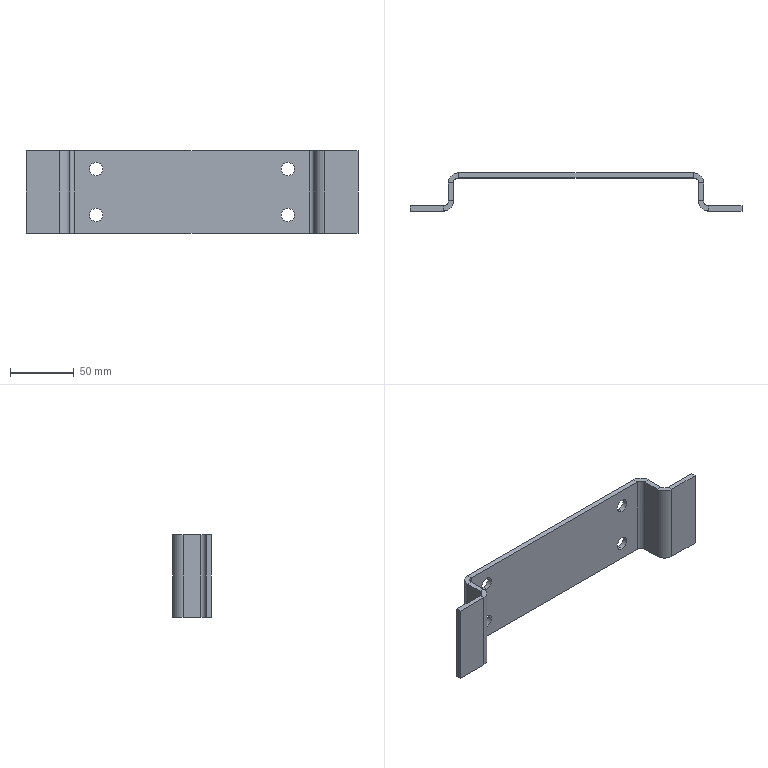Part | SolidWorks | features FlatPattern 1, ICE 1, SMBaseFlange 1, SheetMetal 1 | 1 solid | 46 faces | box 260 x 30 x 64.5 mm | volume 76453 mm3 | plane 30 | cylinder 16 | commonest cylinder face diameters 10.5 x8 8 x4 16 x4
STEP:
#1=CARTESIAN_POINT('',(-75.,-4.,23.25));
#2=VERTEX_POINT('',#1);
#3=CARTESIAN_POINT('',(-75.,-4.,12.75));
#4=VERTEX_POINT('',#3);
#5=CARTESIAN_POINT('',(-75.,-4.,18.));
#6=DIRECTION('',(0.,-1.,0.));
#7=DIRECTION('',(0.,0.,1.));
#8=AXIS2_PLACEMENT_3D('',#5,#6,#7);
#9=CIRCLE('',#8,5.25);
#10=EDGE_CURVE('',#2,#4,#9,.T.);
#11=ORIENTED_EDGE('',*,*,#10,.T.);
#12=CARTESIAN_POINT('',(-75.,0.,12.75));
#13=VERTEX_POINT('',#12);
#14=CARTESIAN_POINT('',(-75.,-30.001,12.75));
#15=DIRECTION('',(0.,1.,0.));
#16=VECTOR('',#15,1000.);
#17=LINE('',#14,#16);
#18=EDGE_CURVE('',#4,#13,#17,.T.);
#19=ORIENTED_EDGE('',*,*,#18,.T.);
#20=CARTESIAN_POINT('',(-75.,0.,23.25));
#21=VERTEX_POINT('',#20);
#22=CARTESIAN_POINT('',(-75.,0.,18.));
#23=DIRECTION('',(0.,1.,0.));
#24=DIRECTION('',(0.,0.,1.));
#25=AXIS2_PLACEMENT_3D('',#22,#23,#24);
#26=CIRCLE('',#25,5.25);
#27=EDGE_CURVE('',#13,#21,#26,.T.);
#28=ORIENTED_EDGE('',*,*,#27,.T.);
#29=CARTESIAN_POINT('',(-75.,-30.001,23.25));
#30=DIRECTION('',(0.,1.,0.));
#31=VECTOR('',#30,1000.);
#32=LINE('',#29,#31);
#33=EDGE_CURVE('',#2,#21,#32,.T.);
#34=ORIENTED_EDGE('',*,*,#33,.F.);
#35=EDGE_LOOP('',(#11,#19,#28,#34));
#36=FACE_OUTER_BOUND('',#35,.T.);
#37=CARTESIAN_POINT('',(-75.,-30.001,18.));
#38=DIRECTION('',(0.,1.,0.));
#39=DIRECTION('',(0.,0.,1.));
#40=AXIS2_PLACEMENT_3D('',#37,#38,#39);
#41=CYLINDRICAL_SURFACE('',#40,5.25);
#42=ADVANCED_FACE('',(#36),#41,.F.);
#43=CARTESIAN_POINT('',(75.,-4.,-12.75));
#44=VERTEX_POINT('',#43);
#45=CARTESIAN_POINT('',(75.,-4.,-23.25));
#46=VERTEX_POINT('',#45);
#47=CARTESIAN_POINT('',(75.,-4.,-18.));
#48=DIRECTION('',(0.,-1.,0.));
#49=DIRECTION('',(0.,0.,1.));
#50=AXIS2_PLACEMENT_3D('',#47,#48,#49);
#51=CIRCLE('',#50,5.25);
#52=EDGE_CURVE('',#44,#46,#51,.T.);
#53=ORIENTED_EDGE('',*,*,#52,.T.);
#54=CARTESIAN_POINT('',(75.,0.,-23.25));
#55=VERTEX_POINT('',#54);
#56=CARTESIAN_POINT('',(75.,-30.001,-23.25));
#57=DIRECTION('',(0.,1.,0.));
#58=VECTOR('',#57,1000.);
#59=LINE('',#56,#58);
#60=EDGE_CURVE('',#46,#55,#59,.T.);
#61=ORIENTED_EDGE('',*,*,#60,.T.);
#62=CARTESIAN_POINT('',(75.,0.,-12.75));
#63=VERTEX_POINT('',#62);
#64=CARTESIAN_POINT('',(75.,0.,-18.));
#65=DIRECTION('',(0.,1.,0.));
#66=DIRECTION('',(0.,0.,1.));
#67=AXIS2_PLACEMENT_3D('',#64,#65,#66);
#68=CIRCLE('',#67,5.25);
#69=EDGE_CURVE('',#55,#63,#68,.T.);
#70=ORIENTED_EDGE('',*,*,#69,.T.);
#71=CARTESIAN_POINT('',(75.,-30.001,-12.75));
#72=DIRECTION('',(0.,1.,0.));
#73=VECTOR('',#72,1000.);
#74=LINE('',#71,#73);
#75=EDGE_CURVE('',#44,#63,#74,.T.);
#76=ORIENTED_EDGE('',*,*,#75,.F.);
#77=EDGE_LOOP('',(#53,#61,#70,#76));
#78=FACE_OUTER_BOUND('',#77,.T.);
#79=CARTESIAN_POINT('',(75.,-30.001,-18.));
#80=DIRECTION('',(0.,1.,0.));
#81=DIRECTION('',(0.,0.,1.));
#82=AXIS2_PLACEMENT_3D('',#79,#80,#81);
#83=CYLINDRICAL_SURFACE('',#82,5.25);
#84=ADVANCED_FACE('',(#78),#83,.F.);
#85=CARTESIAN_POINT('',(75.,-4.,23.25));
#86=VERTEX_POINT('',#85);
#87=CARTESIAN_POINT('',(75.,-4.,12.75));
#88=VERTEX_POINT('',#87);
#89=CARTESIAN_POINT('',(75.,-4.,18.));
#90=DIRECTION('',(0.,-1.,0.));
#91=DIRECTION('',(0.,0.,1.));
#92=AXIS2_PLACEMENT_3D('',#89,#90,#91);
#93=CIRCLE('',#92,5.25);
#94=EDGE_CURVE('',#86,#88,#93,.T.);
#95=ORIENTED_EDGE('',*,*,#94,.T.);
#96=CARTESIAN_POINT('',(75.,0.,12.75));
#97=VERTEX_POINT('',#96);
#98=CARTESIAN_POINT('',(75.,-30.001,12.75));
#99=DIRECTION('',(0.,1.,0.));
#100=VECTOR('',#99,1000.);
#101=LINE('',#98,#100);
#102=EDGE_CURVE('',#88,#97,#101,.T.);
#103=ORIENTED_EDGE('',*,*,#102,.T.);
#104=CARTESIAN_POINT('',(75.,0.,23.25));
#105=VERTEX_POINT('',#104);
#106=CARTESIAN_POINT('',(75.,0.,18.));
#107=DIRECTION('',(0.,1.,0.));
#108=DIRECTION('',(0.,0.,1.));
#109=AXIS2_PLACEMENT_3D('',#106,#107,#108);
#110=CIRCLE('',#109,5.25);
#111=EDGE_CURVE('',#97,#105,#110,.T.);
#112=ORIENTED_EDGE('',*,*,#111,.T.);
#113=CARTESIAN_POINT('',(75.,-30.001,23.25));
#114=DIRECTION('',(0.,1.,0.));
#115=VECTOR('',#114,1000.);
#116=LINE('',#113,#115);
#117=EDGE_CURVE('',#86,#105,#116,.T.);
#118=ORIENTED_EDGE('',*,*,#117,.F.);
#119=EDGE_LOOP('',(#95,#103,#112,#118));
#120=FACE_OUTER_BOUND('',#119,.T.);
#121=CARTESIAN_POINT('',(75.,-30.001,18.));
#122=DIRECTION('',(0.,1.,0.));
#123=DIRECTION('',(0.,0.,1.));
#124=AXIS2_PLACEMENT_3D('',#121,#122,#123);
#125=CYLINDRICAL_SURFACE('',#124,5.25);
#126=ADVANCED_FACE('',(#120),#125,.F.);
#127=CARTESIAN_POINT('',(-75.,-4.,-12.75));
#128=VERTEX_POINT('',#127);
#129=CARTESIAN_POINT('',(-75.,-4.,-23.25));
#130=VERTEX_POINT('',#129);
#131=CARTESIAN_POINT('',(-75.,-4.,-18.));
#132=DIRECTION('',(0.,-1.,0.));
#133=DIRECTION('',(0.,0.,1.));
#134=AXIS2_PLACEMENT_3D('',#131,#132,#133);
#135=CIRCLE('',#134,5.25);
#136=EDGE_CURVE('',#128,#130,#135,.T.);
#137=ORIENTED_EDGE('',*,*,#136,.T.);
#138=CARTESIAN_POINT('',(-75.,0.,-23.25));
#139=VERTEX_POINT('',#138);
#140=CARTESIAN_POINT('',(-75.,-30.001,-23.25));
#141=DIRECTION('',(0.,1.,0.));
#142=VECTOR('',#141,1000.);
#143=LINE('',#140,#142);
#144=EDGE_CURVE('',#130,#139,#143,.T.);
#145=ORIENTED_EDGE('',*,*,#144,.T.);
#146=CARTESIAN_POINT('',(-75.,0.,-12.75));
#147=VERTEX_POINT('',#146);
#148=CARTESIAN_POINT('',(-75.,0.,-18.));
#149=DIRECTION('',(0.,1.,0.));
#150=DIRECTION('',(0.,0.,1.));
#151=AXIS2_PLACEMENT_3D('',#148,#149,#150);
#152=CIRCLE('',#151,5.25);
#153=EDGE_CURVE('',#139,#147,#152,.T.);
#154=ORIENTED_EDGE('',*,*,#153,.T.);
#155=CARTESIAN_POINT('',(-75.,-30.001,-12.75));
#156=DIRECTION('',(0.,1.,0.));
#157=VECTOR('',#156,1000.);
#158=LINE('',#155,#157);
#159=EDGE_CURVE('',#128,#147,#158,.T.);
#160=ORIENTED_EDGE('',*,*,#159,.F.);
#161=EDGE_LOOP('',(#137,#145,#154,#160));
#162=FACE_OUTER_BOUND('',#161,.T.);
#163=CARTESIAN_POINT('',(-75.,-30.001,-18.));
#164=DIRECTION('',(0.,1.,0.));
#165=DIRECTION('',(0.,0.,1.));
#166=AXIS2_PLACEMENT_3D('',#163,#164,#165);
#167=CYLINDRICAL_SURFACE('',#166,5.25);
#168=ADVANCED_FACE('',(#162),#167,.F.);
#169=CARTESIAN_POINT('',(-100.,-22.,32.25));
#170=VERTEX_POINT('',#169);
#171=CARTESIAN_POINT('',(-96.,-22.,32.25));
#172=VERTEX_POINT('',#171);
#173=CARTESIAN_POINT('',(-100.,-22.,32.25));
#174=DIRECTION('',(1.,0.,0.));
#175=VECTOR('',#174,1000.);
#176=LINE('',#173,#175);
#177=EDGE_CURVE('',#170,#172,#176,.T.);
#178=ORIENTED_EDGE('',*,*,#177,.F.);
#179=CARTESIAN_POINT('',(-104.,-26.,32.25));
#180=VERTEX_POINT('',#179);
#181=CARTESIAN_POINT('',(-104.,-22.,32.25));
#182=DIRECTION('',(0.,0.,1.));
#183=DIRECTION('',(-1.,0.,0.));
#184=AXIS2_PLACEMENT_3D('',#181,#182,#183);
#185=CIRCLE('',#184,4.);
#186=EDGE_CURVE('',#180,#170,#185,.T.);
#187=ORIENTED_EDGE('',*,*,#186,.F.);
#188=CARTESIAN_POINT('',(-104.,-30.,32.25));
#189=VERTEX_POINT('',#188);
#190=CARTESIAN_POINT('',(-104.,-30.,32.25));
#191=DIRECTION('',(0.,1.,0.));
#192=VECTOR('',#191,1000.);
#193=LINE('',#190,#192);
#194=EDGE_CURVE('',#189,#180,#193,.T.);
#195=ORIENTED_EDGE('',*,*,#194,.F.);
#196=CARTESIAN_POINT('',(-104.,-22.,32.25));
#197=DIRECTION('',(0.,0.,1.));
#198=DIRECTION('',(1.,0.,0.));
#199=AXIS2_PLACEMENT_3D('',#196,#197,#198);
#200=CIRCLE('',#199,8.);
#201=EDGE_CURVE('',#189,#172,#200,.T.);
#202=ORIENTED_EDGE('',*,*,#201,.T.);
#203=EDGE_LOOP('',(#178,#187,#195,#202));
#204=FACE_OUTER_BOUND('',#203,.T.);
#205=CARTESIAN_POINT('',(-100.,-22.,32.25));
#206=DIRECTION('',(0.,0.,1.));
#207=DIRECTION('',(1.,0.,0.));
#208=AXIS2_PLACEMENT_3D('',#205,#206,#207);
#209=PLANE('',#208);
#210=ADVANCED_FACE('',(#204),#209,.T.);
#211=CARTESIAN_POINT('',(-100.,-8.,32.25));
#212=VERTEX_POINT('',#211);
#213=CARTESIAN_POINT('',(-100.,-26.,32.25));
#214=DIRECTION('',(0.,1.,0.));
#215=VECTOR('',#214,1000.);
#216=LINE('',#213,#215);
#217=EDGE_CURVE('',#170,#212,#216,.T.);
#218=ORIENTED_EDGE('',*,*,#217,.F.);
#219=ORIENTED_EDGE('',*,*,#177,.T.);
#220=CARTESIAN_POINT('',(-96.,-8.,32.25));
#221=VERTEX_POINT('',#220);
#222=CARTESIAN_POINT('',(-96.,-26.,32.25));
#223=DIRECTION('',(0.,1.,0.));
#224=VECTOR('',#223,1000.);
#225=LINE('',#222,#224);
#226=EDGE_CURVE('',#172,#221,#225,.T.);
#227=ORIENTED_EDGE('',*,*,#226,.T.);
#228=CARTESIAN_POINT('',(-96.,-8.,32.25));
#229=DIRECTION('',(-1.,0.,0.));
#230=VECTOR('',#229,1000.);
#231=LINE('',#228,#230);
#232=EDGE_CURVE('',#221,#212,#231,.T.);
#233=ORIENTED_EDGE('',*,*,#232,.T.);
#234=EDGE_LOOP('',(#218,#219,#227,#233));
#235=FACE_OUTER_BOUND('',#234,.T.);
#236=CARTESIAN_POINT('',(-104.,-30.,32.25));
#237=DIRECTION('',(0.,0.,1.));
#238=DIRECTION('',(1.,0.,0.));
#239=AXIS2_PLACEMENT_3D('',#236,#237,#238);
#240=PLANE('',#239);
#241=ADVANCED_FACE('',(#235),#240,.T.);
#242=CARTESIAN_POINT('',(-104.,-26.,-32.25));
#243=VERTEX_POINT('',#242);
#244=CARTESIAN_POINT('',(-104.,-30.,-32.25));
#245=VERTEX_POINT('',#244);
#246=CARTESIAN_POINT('',(-104.,-26.,-32.25));
#247=DIRECTION('',(0.,-1.,0.));
#248=VECTOR('',#247,1000.);
#249=LINE('',#246,#248);
#250=EDGE_CURVE('',#243,#245,#249,.T.);
#251=ORIENTED_EDGE('',*,*,#250,.F.);
#252=CARTESIAN_POINT('',(-100.,-22.,-32.25));
#253=VERTEX_POINT('',#252);
#254=CARTESIAN_POINT('',(-104.,-22.,-32.25));
#255=DIRECTION('',(0.,0.,1.));
#256=DIRECTION('',(-1.,0.,0.));
#257=AXIS2_PLACEMENT_3D('',#254,#255,#256);
#258=CIRCLE('',#257,4.);
#259=EDGE_CURVE('',#243,#253,#258,.T.);
#260=ORIENTED_EDGE('',*,*,#259,.T.);
#261=CARTESIAN_POINT('',(-96.,-22.,-32.25));
#262=VERTEX_POINT('',#261);
#263=CARTESIAN_POINT('',(-96.,-22.,-32.25));
#264=DIRECTION('',(-1.,0.,0.));
#265=VECTOR('',#264,1000.);
#266=LINE('',#263,#265);
#267=EDGE_CURVE('',#262,#253,#266,.T.);
#268=ORIENTED_EDGE('',*,*,#267,.F.);
#269=CARTESIAN_POINT('',(-104.,-22.,-32.25));
#270=DIRECTION('',(0.,0.,1.));
#271=DIRECTION('',(1.,0.,0.));
#272=AXIS2_PLACEMENT_3D('',#269,#270,#271);
#273=CIRCLE('',#272,8.);
#274=EDGE_CURVE('',#245,#262,#273,.T.);
#275=ORIENTED_EDGE('',*,*,#274,.F.);
#276=EDGE_LOOP('',(#251,#260,#268,#275));
#277=FACE_OUTER_BOUND('',#276,.T.);
#278=CARTESIAN_POINT('',(-104.,-26.,-32.25));
#279=DIRECTION('',(0.,0.,-1.));
#280=DIRECTION('',(-1.,0.,0.));
#281=AXIS2_PLACEMENT_3D('',#278,#279,#280);
#282=PLANE('',#281);
#283=ADVANCED_FACE('',(#277),#282,.T.);
#284=CARTESIAN_POINT('',(-130.,-26.,-32.25));
#285=VERTEX_POINT('',#284);
#286=CARTESIAN_POINT('',(-130.,-26.,-32.25));
#287=DIRECTION('',(1.,0.,0.));
#288=VECTOR('',#287,1000.);
#289=LINE('',#286,#288);
#290=EDGE_CURVE('',#285,#243,#289,.T.);
#291=ORIENTED_EDGE('',*,*,#290,.T.);
#292=ORIENTED_EDGE('',*,*,#250,.T.);
#293=CARTESIAN_POINT('',(-130.,-30.,-32.25));
#294=VERTEX_POINT('',#293);
#295=CARTESIAN_POINT('',(-130.,-30.,-32.25));
#296=DIRECTION('',(1.,0.,0.));
#297=VECTOR('',#296,1000.);
#298=LINE('',#295,#297);
#299=EDGE_CURVE('',#294,#245,#298,.T.);
#300=ORIENTED_EDGE('',*,*,#299,.F.);
#301=CARTESIAN_POINT('',(-130.,-30.,-32.25));
#302=DIRECTION('',(0.,1.,0.));
#303=VECTOR('',#302,1000.);
#304=LINE('',#301,#303);
#305=EDGE_CURVE('',#294,#285,#304,.T.);
#306=ORIENTED_EDGE('',*,*,#305,.T.);
#307=EDGE_LOOP('',(#291,#292,#300,#306));
#308=FACE_OUTER_BOUND('',#307,.T.);
#309=CARTESIAN_POINT('',(-96.,-22.,-32.25));
#310=DIRECTION('',(0.,0.,-1.));
#311=DIRECTION('',(-1.,0.,0.));
#312=AXIS2_PLACEMENT_3D('',#309,#310,#311);
#313=PLANE('',#312);
#314=ADVANCED_FACE('',(#308),#313,.T.);
#315=CARTESIAN_POINT('',(-92.,0.,32.25));
#316=VERTEX_POINT('',#315);
#317=CARTESIAN_POINT('',(-92.,-4.,32.25));
#318=VERTEX_POINT('',#317);
#319=CARTESIAN_POINT('',(-92.,0.,32.25));
#320=DIRECTION('',(0.,-1.,0.));
#321=VECTOR('',#320,1000.);
#322=LINE('',#319,#321);
#323=EDGE_CURVE('',#316,#318,#322,.T.);
#324=ORIENTED_EDGE('',*,*,#323,.F.);
#325=CARTESIAN_POINT('',(-92.,-8.,32.25));
#326=DIRECTION('',(0.,0.,-1.));
#327=DIRECTION('',(1.,0.,0.));
#328=AXIS2_PLACEMENT_3D('',#325,#326,#327);
#329=CIRCLE('',#328,8.);
#330=EDGE_CURVE('',#212,#316,#329,.T.);
#331=ORIENTED_EDGE('',*,*,#330,.F.);
#332=ORIENTED_EDGE('',*,*,#232,.F.);
#333=CARTESIAN_POINT('',(-92.,-8.,32.25));
#334=DIRECTION('',(0.,0.,-1.));
#335=DIRECTION('',(1.,0.,0.));
#336=AXIS2_PLACEMENT_3D('',#333,#334,#335);
#337=CIRCLE('',#336,4.);
#338=EDGE_CURVE('',#221,#318,#337,.T.);
#339=ORIENTED_EDGE('',*,*,#338,.T.);
#340=EDGE_LOOP('',(#324,#331,#332,#339));
#341=FACE_OUTER_BOUND('',#340,.T.);
#342=CARTESIAN_POINT('',(-92.,0.,32.25));
#343=DIRECTION('',(0.,0.,1.));
#344=DIRECTION('',(1.,0.,0.));
#345=AXIS2_PLACEMENT_3D('',#342,#343,#344);
#346=PLANE('',#345);
#347=ADVANCED_FACE('',(#341),#346,.T.);
#348=CARTESIAN_POINT('',(92.,0.,32.25));
#349=VERTEX_POINT('',#348);
#350=CARTESIAN_POINT('',(-100.,0.,32.25));
#351=DIRECTION('',(1.,0.,0.));
#352=VECTOR('',#351,1000.);
#353=LINE('',#350,#352);
#354=EDGE_CURVE('',#316,#349,#353,.T.);
#355=ORIENTED_EDGE('',*,*,#354,.F.);
#356=ORIENTED_EDGE('',*,*,#323,.T.);
#357=CARTESIAN_POINT('',(92.,-4.,32.25));
#358=VERTEX_POINT('',#357);
#359=CARTESIAN_POINT('',(-100.,-4.,32.25));
#360=DIRECTION('',(1.,0.,0.));
#361=VECTOR('',#360,1000.);
#362=LINE('',#359,#361);
#363=EDGE_CURVE('',#318,#358,#362,.T.);
#364=ORIENTED_EDGE('',*,*,#363,.T.);
#365=CARTESIAN_POINT('',(92.,-4.,32.25));
#366=DIRECTION('',(0.,1.,0.));
#367=VECTOR('',#366,1000.);
#368=LINE('',#365,#367);
#369=EDGE_CURVE('',#358,#349,#368,.T.);
#370=ORIENTED_EDGE('',*,*,#369,.T.);
#371=EDGE_LOOP('',(#355,#356,#364,#370));
#372=FACE_OUTER_BOUND('',#371,.T.);
#373=CARTESIAN_POINT('',(-96.,-8.,32.25));
#374=DIRECTION('',(0.,0.,1.));
#375=DIRECTION('',(1.,0.,0.));
#376=AXIS2_PLACEMENT_3D('',#373,#374,#375);
#377=PLANE('',#376);
#378=ADVANCED_FACE('',(#372),#377,.T.);
#379=CARTESIAN_POINT('',(-100.,-8.,-32.25));
#380=VERTEX_POINT('',#379);
#381=CARTESIAN_POINT('',(-96.,-8.,-32.25));
#382=VERTEX_POINT('',#381);
#383=CARTESIAN_POINT('',(-100.,-8.,-32.25));
#384=DIRECTION('',(1.,0.,0.));
#385=VECTOR('',#384,1000.);
#386=LINE('',#383,#385);
#387=EDGE_CURVE('',#380,#382,#386,.T.);
#388=ORIENTED_EDGE('',*,*,#387,.F.);
#389=CARTESIAN_POINT('',(-92.,0.,-32.25));
#390=VERTEX_POINT('',#389);
#391=CARTESIAN_POINT('',(-92.,-8.,-32.25));
#392=DIRECTION('',(0.,0.,-1.));
#393=DIRECTION('',(1.,0.,0.));
#394=AXIS2_PLACEMENT_3D('',#391,#392,#393);
#395=CIRCLE('',#394,8.);
#396=EDGE_CURVE('',#380,#390,#395,.T.);
#397=ORIENTED_EDGE('',*,*,#396,.T.);
#398=CARTESIAN_POINT('',(-92.,-4.,-32.25));
#399=VERTEX_POINT('',#398);
#400=CARTESIAN_POINT('',(-92.,-4.,-32.25));
#401=DIRECTION('',(0.,1.,0.));
#402=VECTOR('',#401,1000.);
#403=LINE('',#400,#402);
#404=EDGE_CURVE('',#399,#390,#403,.T.);
#405=ORIENTED_EDGE('',*,*,#404,.F.);
#406=CARTESIAN_POINT('',(-92.,-8.,-32.25));
#407=DIRECTION('',(0.,0.,-1.));
#408=DIRECTION('',(1.,0.,0.));
#409=AXIS2_PLACEMENT_3D('',#406,#407,#408);
#410=CIRCLE('',#409,4.);
#411=EDGE_CURVE('',#382,#399,#410,.T.);
#412=ORIENTED_EDGE('',*,*,#411,.F.);
#413=EDGE_LOOP('',(#388,#397,#405,#412));
#414=FACE_OUTER_BOUND('',#413,.T.);
#415=CARTESIAN_POINT('',(-100.,-8.,-32.25));
#416=DIRECTION('',(0.,0.,-1.));
#417=DIRECTION('',(-1.,0.,0.));
#418=AXIS2_PLACEMENT_3D('',#415,#416,#417);
#419=PLANE('',#418);
#420=ADVANCED_FACE('',(#414),#419,.T.);
#421=CARTESIAN_POINT('',(-100.,-26.,-32.25));
#422=DIRECTION('',(0.,1.,0.));
#423=VECTOR('',#422,1000.);
#424=LINE('',#421,#423);
#425=EDGE_CURVE('',#253,#380,#424,.T.);
#426=ORIENTED_EDGE('',*,*,#425,.T.);
#427=ORIENTED_EDGE('',*,*,#387,.T.);
#428=CARTESIAN_POINT('',(-96.,-26.,-32.25));
#429=DIRECTION('',(0.,1.,0.));
#430=VECTOR('',#429,1000.);
#431=LINE('',#428,#430);
#432=EDGE_CURVE('',#262,#382,#431,.T.);
#433=ORIENTED_EDGE('',*,*,#432,.F.);
#434=ORIENTED_EDGE('',*,*,#267,.T.);
#435=EDGE_LOOP('',(#426,#427,#433,#434));
#436=FACE_OUTER_BOUND('',#435,.T.);
#437=CARTESIAN_POINT('',(-92.,-4.,-32.25));
#438=DIRECTION('',(0.,0.,-1.));
#439=DIRECTION('',(-1.,0.,0.));
#440=AXIS2_PLACEMENT_3D('',#437,#438,#439);
#441=PLANE('',#440);
#442=ADVANCED_FACE('',(#436),#441,.T.);
#443=CARTESIAN_POINT('',(100.,-8.,32.25));
#444=VERTEX_POINT('',#443);
#445=CARTESIAN_POINT('',(96.,-8.,32.25));
#446=VERTEX_POINT('',#445);
#447=CARTESIAN_POINT('',(100.,-8.,32.25));
#448=DIRECTION('',(-1.,0.,0.));
#449=VECTOR('',#448,1000.);
#450=LINE('',#447,#449);
#451=EDGE_CURVE('',#444,#446,#450,.T.);
#452=ORIENTED_EDGE('',*,*,#451,.F.);
#453=CARTESIAN_POINT('',(92.,-8.,32.25));
#454=DIRECTION('',(0.,0.,-1.));
#455=DIRECTION('',(1.,0.,0.));
#456=AXIS2_PLACEMENT_3D('',#453,#454,#455);
#457=CIRCLE('',#456,8.);
#458=EDGE_CURVE('',#349,#444,#457,.T.);
#459=ORIENTED_EDGE('',*,*,#458,.F.);
#460=ORIENTED_EDGE('',*,*,#369,.F.);
#461=CARTESIAN_POINT('',(92.,-8.,32.25));
#462=DIRECTION('',(0.,0.,-1.));
#463=DIRECTION('',(1.,0.,0.));
#464=AXIS2_PLACEMENT_3D('',#461,#462,#463);
#465=CIRCLE('',#464,4.);
#466=EDGE_CURVE('',#358,#446,#465,.T.);
#467=ORIENTED_EDGE('',*,*,#466,.T.);
#468=EDGE_LOOP('',(#452,#459,#460,#467));
#469=FACE_OUTER_BOUND('',#468,.T.);
#470=CARTESIAN_POINT('',(100.,-8.,32.25));
#471=DIRECTION('',(0.,0.,1.));
#472=DIRECTION('',(1.,0.,0.));
#473=AXIS2_PLACEMENT_3D('',#470,#471,#472);
#474=PLANE('',#473);
#475=ADVANCED_FACE('',(#469),#474,.T.);
#476=CARTESIAN_POINT('',(100.,-22.,32.25));
#477=VERTEX_POINT('',#476);
#478=CARTESIAN_POINT('',(100.,0.,32.25));
#479=DIRECTION('',(0.,-1.,0.));
#480=VECTOR('',#479,1000.);
#481=LINE('',#478,#480);
#482=EDGE_CURVE('',#444,#477,#481,.T.);
#483=ORIENTED_EDGE('',*,*,#482,.F.);
#484=ORIENTED_EDGE('',*,*,#451,.T.);
#485=CARTESIAN_POINT('',(96.,-22.,32.25));
#486=VERTEX_POINT('',#485);
#487=CARTESIAN_POINT('',(96.,0.,32.25));
#488=DIRECTION('',(0.,-1.,0.));
#489=VECTOR('',#488,1000.);
#490=LINE('',#487,#489);
#491=EDGE_CURVE('',#446,#486,#490,.T.);
#492=ORIENTED_EDGE('',*,*,#491,.T.);
#493=CARTESIAN_POINT('',(96.,-22.,32.25));
#494=DIRECTION('',(1.,0.,0.));
#495=VECTOR('',#494,1000.);
#496=LINE('',#493,#495);
#497=EDGE_CURVE('',#486,#477,#496,.T.);
#498=ORIENTED_EDGE('',*,*,#497,.T.);
#499=EDGE_LOOP('',(#483,#484,#492,#498));
#500=FACE_OUTER_BOUND('',#499,.T.);
#501=CARTESIAN_POINT('',(92.,-4.,32.25));
#502=DIRECTION('',(0.,0.,1.));
#503=DIRECTION('',(1.,0.,0.));
#504=AXIS2_PLACEMENT_3D('',#501,#502,#503);
#505=PLANE('',#504);
#506=ADVANCED_FACE('',(#500),#505,.T.);
#507=CARTESIAN_POINT('',(92.,0.,-32.25));
#508=VERTEX_POINT('',#507);
#509=CARTESIAN_POINT('',(92.,-4.,-32.25));
#510=VERTEX_POINT('',#509);
#511=CARTESIAN_POINT('',(92.,0.,-32.25));
#512=DIRECTION('',(0.,-1.,0.));
#513=VECTOR('',#512,1000.);
#514=LINE('',#511,#513);
#515=EDGE_CURVE('',#508,#510,#514,.T.);
#516=ORIENTED_EDGE('',*,*,#515,.F.);
#517=CARTESIAN_POINT('',(100.,-8.,-32.25));
#518=VERTEX_POINT('',#517);
#519=CARTESIAN_POINT('',(92.,-8.,-32.25));
#520=DIRECTION('',(0.,0.,-1.));
#521=DIRECTION('',(1.,0.,0.));
#522=AXIS2_PLACEMENT_3D('',#519,#520,#521);
#523=CIRCLE('',#522,8.);
#524=EDGE_CURVE('',#508,#518,#523,.T.);
#525=ORIENTED_EDGE('',*,*,#524,.T.);
#526=CARTESIAN_POINT('',(96.,-8.,-32.25));
#527=VERTEX_POINT('',#526);
#528=CARTESIAN_POINT('',(96.,-8.,-32.25));
#529=DIRECTION('',(1.,0.,0.));
#530=VECTOR('',#529,1000.);
#531=LINE('',#528,#530);
#532=EDGE_CURVE('',#527,#518,#531,.T.);
#533=ORIENTED_EDGE('',*,*,#532,.F.);
#534=CARTESIAN_POINT('',(92.,-8.,-32.25));
#535=DIRECTION('',(0.,0.,-1.));
#536=DIRECTION('',(1.,0.,0.));
#537=AXIS2_PLACEMENT_3D('',#534,#535,#536);
#538=CIRCLE('',#537,4.);
#539=EDGE_CURVE('',#510,#527,#538,.T.);
#540=ORIENTED_EDGE('',*,*,#539,.F.);
#541=EDGE_LOOP('',(#516,#525,#533,#540));
#542=FACE_OUTER_BOUND('',#541,.T.);
#543=CARTESIAN_POINT('',(92.,0.,-32.25));
#544=DIRECTION('',(0.,0.,-1.));
#545=DIRECTION('',(-1.,0.,0.));
#546=AXIS2_PLACEMENT_3D('',#543,#544,#545);
#547=PLANE('',#546);
#548=ADVANCED_FACE('',(#542),#547,.T.);
#549=CARTESIAN_POINT('',(-100.,0.,-32.25));
#550=DIRECTION('',(1.,0.,0.));
#551=VECTOR('',#550,1000.);
#552=LINE('',#549,#551);
#553=EDGE_CURVE('',#390,#508,#552,.T.);
#554=ORIENTED_EDGE('',*,*,#553,.T.);
#555=ORIENTED_EDGE('',*,*,#515,.T.);
#556=CARTESIAN_POINT('',(-100.,-4.,-32.25));
#557=DIRECTION('',(1.,0.,0.));
#558=VECTOR('',#557,1000.);
#559=LINE('',#556,#558);
#560=EDGE_CURVE('',#399,#510,#559,.T.);
#561=ORIENTED_EDGE('',*,*,#560,.F.);
#562=ORIENTED_EDGE('',*,*,#404,.T.);
#563=EDGE_LOOP('',(#554,#555,#561,#562));
#564=FACE_OUTER_BOUND('',#563,.T.);
#565=CARTESIAN_POINT('',(96.,-8.,-32.25));
#566=DIRECTION('',(0.,0.,-1.));
#567=DIRECTION('',(-1.,0.,0.));
#568=AXIS2_PLACEMENT_3D('',#565,#566,#567);
#569=PLANE('',#568);
#570=ADVANCED_FACE('',(#564),#569,.T.);
#571=CARTESIAN_POINT('',(104.,-26.,32.25));
#572=VERTEX_POINT('',#571);
#573=CARTESIAN_POINT('',(104.,-30.,32.25));
#574=VERTEX_POINT('',#573);
#575=CARTESIAN_POINT('',(104.,-26.,32.25));
#576=DIRECTION('',(0.,-1.,0.));
#577=VECTOR('',#576,1000.);
#578=LINE('',#575,#577);
#579=EDGE_CURVE('',#572,#574,#578,.T.);
#580=ORIENTED_EDGE('',*,*,#579,.F.);
#581=CARTESIAN_POINT('',(104.,-22.,32.25));
#582=DIRECTION('',(0.,0.,1.));
#583=DIRECTION('',(-1.,0.,0.));
#584=AXIS2_PLACEMENT_3D('',#581,#582,#583);
#585=CIRCLE('',#584,4.);
#586=EDGE_CURVE('',#477,#572,#585,.T.);
#587=ORIENTED_EDGE('',*,*,#586,.F.);
#588=ORIENTED_EDGE('',*,*,#497,.F.);
#589=CARTESIAN_POINT('',(104.,-22.,32.25));
#590=DIRECTION('',(0.,0.,1.));
#591=DIRECTION('',(1.,0.,0.));
#592=AXIS2_PLACEMENT_3D('',#589,#590,#591);
#593=CIRCLE('',#592,8.);
#594=EDGE_CURVE('',#486,#574,#593,.T.);
#595=ORIENTED_EDGE('',*,*,#594,.T.);
#596=EDGE_LOOP('',(#580,#587,#588,#595));
#597=FACE_OUTER_BOUND('',#596,.T.);
#598=CARTESIAN_POINT('',(104.,-26.,32.25));
#599=DIRECTION('',(0.,0.,1.));
#600=DIRECTION('',(1.,0.,0.));
#601=AXIS2_PLACEMENT_3D('',#598,#599,#600);
#602=PLANE('',#601);
#603=ADVANCED_FACE('',(#597),#602,.T.);
#604=CARTESIAN_POINT('',(130.,-26.,32.25));
#605=VERTEX_POINT('',#604);
#606=CARTESIAN_POINT('',(100.,-26.,32.25));
#607=DIRECTION('',(1.,0.,0.));
#608=VECTOR('',#607,1000.);
#609=LINE('',#606,#608);
#610=EDGE_CURVE('',#572,#605,#609,.T.);
#611=ORIENTED_EDGE('',*,*,#610,.F.);
#612=ORIENTED_EDGE('',*,*,#579,.T.);
#613=CARTESIAN_POINT('',(130.,-30.,32.25));
#614=VERTEX_POINT('',#613);
#615=CARTESIAN_POINT('',(100.,-30.,32.25));
#616=DIRECTION('',(1.,0.,0.));
#617=VECTOR('',#616,1000.);
#618=LINE('',#615,#617);
#619=EDGE_CURVE('',#574,#614,#618,.T.);
#620=ORIENTED_EDGE('',*,*,#619,.T.);
#621=CARTESIAN_POINT('',(130.,-26.,32.25));
#622=DIRECTION('',(0.,-1.,0.));
#623=VECTOR('',#622,1000.);
#624=LINE('',#621,#623);
#625=EDGE_CURVE('',#605,#614,#624,.T.);
#626=ORIENTED_EDGE('',*,*,#625,.F.);
#627=EDGE_LOOP('',(#611,#612,#620,#626));
#628=FACE_OUTER_BOUND('',#627,.T.);
#629=CARTESIAN_POINT('',(96.,-22.,32.25));
#630=DIRECTION('',(0.,0.,1.));
#631=DIRECTION('',(1.,0.,0.));
#632=AXIS2_PLACEMENT_3D('',#629,#630,#631);
#633=PLANE('',#632);
#634=ADVANCED_FACE('',(#628),#633,.T.);
#635=CARTESIAN_POINT('',(100.,-22.,-32.25));
#636=VERTEX_POINT('',#635);
#637=CARTESIAN_POINT('',(96.,-22.,-32.25));
#638=VERTEX_POINT('',#637);
#639=CARTESIAN_POINT('',(100.,-22.,-32.25));
#640=DIRECTION('',(-1.,0.,0.));
#641=VECTOR('',#640,1000.);
#642=LINE('',#639,#641);
#643=EDGE_CURVE('',#636,#638,#642,.T.);
#644=ORIENTED_EDGE('',*,*,#643,.F.);
#645=CARTESIAN_POINT('',(104.,-26.,-32.25));
#646=VERTEX_POINT('',#645);
#647=CARTESIAN_POINT('',(104.,-22.,-32.25));
#648=DIRECTION('',(0.,0.,1.));
#649=DIRECTION('',(-1.,0.,0.));
#650=AXIS2_PLACEMENT_3D('',#647,#648,#649);
#651=CIRCLE('',#650,4.);
#652=EDGE_CURVE('',#636,#646,#651,.T.);
#653=ORIENTED_EDGE('',*,*,#652,.T.);
#654=CARTESIAN_POINT('',(104.,-30.,-32.25));
#655=VERTEX_POINT('',#654);
#656=CARTESIAN_POINT('',(104.,-30.,-32.25));
#657=DIRECTION('',(0.,1.,0.));
#658=VECTOR('',#657,1000.);
#659=LINE('',#656,#658);
#660=EDGE_CURVE('',#655,#646,#659,.T.);
#661=ORIENTED_EDGE('',*,*,#660,.F.);
#662=CARTESIAN_POINT('',(104.,-22.,-32.25));
#663=DIRECTION('',(0.,0.,1.));
#664=DIRECTION('',(1.,0.,0.));
#665=AXIS2_PLACEMENT_3D('',#662,#663,#664);
#666=CIRCLE('',#665,8.);
#667=EDGE_CURVE('',#638,#655,#666,.T.);
#668=ORIENTED_EDGE('',*,*,#667,.F.);
#669=EDGE_LOOP('',(#644,#653,#661,#668));
#670=FACE_OUTER_BOUND('',#669,.T.);
#671=CARTESIAN_POINT('',(100.,-22.,-32.25));
#672=DIRECTION('',(0.,0.,-1.));
#673=DIRECTION('',(-1.,0.,0.));
#674=AXIS2_PLACEMENT_3D('',#671,#672,#673);
#675=PLANE('',#674);
#676=ADVANCED_FACE('',(#670),#675,.T.);
#677=CARTESIAN_POINT('',(100.,0.,-32.25));
#678=DIRECTION('',(0.,-1.,0.));
#679=VECTOR('',#678,1000.);
#680=LINE('',#677,#679);
#681=EDGE_CURVE('',#518,#636,#680,.T.);
#682=ORIENTED_EDGE('',*,*,#681,.T.);
#683=ORIENTED_EDGE('',*,*,#643,.T.);
#684=CARTESIAN_POINT('',(96.,0.,-32.25));
#685=DIRECTION('',(0.,-1.,0.));
#686=VECTOR('',#685,1000.);
#687=LINE('',#684,#686);
#688=EDGE_CURVE('',#527,#638,#687,.T.);
#689=ORIENTED_EDGE('',*,*,#688,.F.);
#690=ORIENTED_EDGE('',*,*,#532,.T.);
#691=EDGE_LOOP('',(#682,#683,#689,#690));
#692=FACE_OUTER_BOUND('',#691,.T.);
#693=CARTESIAN_POINT('',(104.,-30.,-32.25));
#694=DIRECTION('',(0.,0.,-1.));
#695=DIRECTION('',(-1.,0.,0.));
#696=AXIS2_PLACEMENT_3D('',#693,#694,#695);
#697=PLANE('',#696);
#698=ADVANCED_FACE('',(#692),#697,.T.);
#699=CARTESIAN_POINT('',(130.,-30.,-32.25));
#700=VERTEX_POINT('',#699);
#701=CARTESIAN_POINT('',(100.,-30.,-32.25));
#702=DIRECTION('',(1.,0.,0.));
#703=VECTOR('',#702,1000.);
#704=LINE('',#701,#703);
#705=EDGE_CURVE('',#655,#700,#704,.T.);
#706=ORIENTED_EDGE('',*,*,#705,.T.);
#707=CARTESIAN_POINT('',(130.,-30.,32.25));
#708=DIRECTION('',(0.,0.,-1.));
#709=VECTOR('',#708,1000.);
#710=LINE('',#707,#709);
#711=EDGE_CURVE('',#614,#700,#710,.T.);
#712=ORIENTED_EDGE('',*,*,#711,.F.);
#713=ORIENTED_EDGE('',*,*,#619,.F.);
#714=CARTESIAN_POINT('',(104.,-30.,32.25));
#715=DIRECTION('',(0.,0.,-1.));
#716=VECTOR('',#715,1000.);
#717=LINE('',#714,#716);
#718=EDGE_CURVE('',#574,#655,#717,.T.);
#719=ORIENTED_EDGE('',*,*,#718,.T.);
#720=EDGE_LOOP('',(#706,#712,#713,#719));
#721=FACE_OUTER_BOUND('',#720,.T.);
#722=CARTESIAN_POINT('',(100.,-30.,32.25));
#723=DIRECTION('',(0.,1.,0.));
#724=DIRECTION('',(0.,0.,1.));
#725=AXIS2_PLACEMENT_3D('',#722,#723,#724);
#726=PLANE('',#725);
#727=ADVANCED_FACE('',(#721),#726,.F.);
#728=CARTESIAN_POINT('',(130.,-26.,-32.25));
#729=VERTEX_POINT('',#728);
#730=CARTESIAN_POINT('',(130.,-26.,-32.25));
#731=DIRECTION('',(0.,-1.,0.));
#732=VECTOR('',#731,1000.);
#733=LINE('',#730,#732);
#734=EDGE_CURVE('',#729,#700,#733,.T.);
#735=ORIENTED_EDGE('',*,*,#734,.F.);
#736=CARTESIAN_POINT('',(130.,-26.,32.25));
#737=DIRECTION('',(0.,0.,-1.));
#738=VECTOR('',#737,1000.);
#739=LINE('',#736,#738);
#740=EDGE_CURVE('',#605,#729,#739,.T.);
#741=ORIENTED_EDGE('',*,*,#740,.F.);
#742=ORIENTED_EDGE('',*,*,#625,.T.);
#743=ORIENTED_EDGE('',*,*,#711,.T.);
#744=EDGE_LOOP('',(#735,#741,#742,#743));
#745=FACE_OUTER_BOUND('',#744,.T.);
#746=CARTESIAN_POINT('',(130.,-26.,32.25));
#747=DIRECTION('',(1.,0.,0.));
#748=DIRECTION('',(0.,0.,-1.));
#749=AXIS2_PLACEMENT_3D('',#746,#747,#748);
#750=PLANE('',#749);
#751=ADVANCED_FACE('',(#745),#750,.T.);
#752=CARTESIAN_POINT('',(100.,-26.,-32.25));
#753=DIRECTION('',(1.,0.,0.));
#754=VECTOR('',#753,1000.);
#755=LINE('',#752,#754);
#756=EDGE_CURVE('',#646,#729,#755,.T.);
#757=ORIENTED_EDGE('',*,*,#756,.F.);
#758=CARTESIAN_POINT('',(104.,-26.,32.25));
#759=DIRECTION('',(0.,0.,-1.));
#760=VECTOR('',#759,1000.);
#761=LINE('',#758,#760);
#762=EDGE_CURVE('',#572,#646,#761,.T.);
#763=ORIENTED_EDGE('',*,*,#762,.F.);
#764=ORIENTED_EDGE('',*,*,#610,.T.);
#765=ORIENTED_EDGE('',*,*,#740,.T.);
#766=EDGE_LOOP('',(#757,#763,#764,#765));
#767=FACE_OUTER_BOUND('',#766,.T.);
#768=CARTESIAN_POINT('',(100.,-26.,32.25));
#769=DIRECTION('',(0.,1.,0.));
#770=DIRECTION('',(0.,0.,1.));
#771=AXIS2_PLACEMENT_3D('',#768,#769,#770);
#772=PLANE('',#771);
#773=ADVANCED_FACE('',(#767),#772,.T.);
#774=ORIENTED_EDGE('',*,*,#652,.F.);
#775=CARTESIAN_POINT('',(100.,-22.,32.25));
#776=DIRECTION('',(0.,0.,-1.));
#777=VECTOR('',#776,1000.);
#778=LINE('',#775,#777);
#779=EDGE_CURVE('',#477,#636,#778,.T.);
#780=ORIENTED_EDGE('',*,*,#779,.F.);
#781=ORIENTED_EDGE('',*,*,#586,.T.);
#782=ORIENTED_EDGE('',*,*,#762,.T.);
#783=EDGE_LOOP('',(#774,#780,#781,#782));
#784=FACE_OUTER_BOUND('',#783,.T.);
#785=CARTESIAN_POINT('',(104.,-22.,32.25));
#786=DIRECTION('',(0.,0.,-1.));
#787=DIRECTION('',(-1.,0.,0.));
#788=AXIS2_PLACEMENT_3D('',#785,#786,#787);
#789=CYLINDRICAL_SURFACE('',#788,4.);
#790=ADVANCED_FACE('',(#784),#789,.F.);
#791=ORIENTED_EDGE('',*,*,#681,.F.);
#792=CARTESIAN_POINT('',(100.,-8.,32.25));
#793=DIRECTION('',(0.,0.,-1.));
#794=VECTOR('',#793,1000.);
#795=LINE('',#792,#794);
#796=EDGE_CURVE('',#444,#518,#795,.T.);
#797=ORIENTED_EDGE('',*,*,#796,.F.);
#798=ORIENTED_EDGE('',*,*,#482,.T.);
#799=ORIENTED_EDGE('',*,*,#779,.T.);
#800=EDGE_LOOP('',(#791,#797,#798,#799));
#801=FACE_OUTER_BOUND('',#800,.T.);
#802=CARTESIAN_POINT('',(100.,0.,32.25));
#803=DIRECTION('',(1.,0.,0.));
#804=DIRECTION('',(0.,0.,-1.));
#805=AXIS2_PLACEMENT_3D('',#802,#803,#804);
#806=PLANE('',#805);
#807=ADVANCED_FACE('',(#801),#806,.T.);
#808=ORIENTED_EDGE('',*,*,#524,.F.);
#809=CARTESIAN_POINT('',(92.,0.,32.25));
#810=DIRECTION('',(0.,0.,-1.));
#811=VECTOR('',#810,1000.);
#812=LINE('',#809,#811);
#813=EDGE_CURVE('',#349,#508,#812,.T.);
#814=ORIENTED_EDGE('',*,*,#813,.F.);
#815=ORIENTED_EDGE('',*,*,#458,.T.);
#816=ORIENTED_EDGE('',*,*,#796,.T.);
#817=EDGE_LOOP('',(#808,#814,#815,#816));
#818=FACE_OUTER_BOUND('',#817,.T.);
#819=CARTESIAN_POINT('',(92.,-8.,32.25));
#820=DIRECTION('',(0.,0.,-1.));
#821=DIRECTION('',(-1.,0.,0.));
#822=AXIS2_PLACEMENT_3D('',#819,#820,#821);
#823=CYLINDRICAL_SURFACE('',#822,8.);
#824=ADVANCED_FACE('',(#818),#823,.T.);
#825=CARTESIAN_POINT('',(-75.,0.,18.));
#826=DIRECTION('',(0.,1.,0.));
#827=DIRECTION('',(0.,0.,1.));
#828=AXIS2_PLACEMENT_3D('',#825,#826,#827);
#829=CIRCLE('',#828,5.25);
#830=EDGE_CURVE('',#21,#13,#829,.T.);
#831=ORIENTED_EDGE('',*,*,#830,.F.);
#832=ORIENTED_EDGE('',*,*,#27,.F.);
#833=EDGE_LOOP('',(#831,#832));
#834=FACE_BOUND('',#833,.T.);
#835=CARTESIAN_POINT('',(75.,0.,-18.));
#836=DIRECTION('',(0.,1.,0.));
#837=DIRECTION('',(0.,0.,1.));
#838=AXIS2_PLACEMENT_3D('',#835,#836,#837);
#839=CIRCLE('',#838,5.25);
#840=EDGE_CURVE('',#63,#55,#839,.T.);
#841=ORIENTED_EDGE('',*,*,#840,.F.);
#842=ORIENTED_EDGE('',*,*,#69,.F.);
#843=EDGE_LOOP('',(#841,#842));
#844=FACE_BOUND('',#843,.T.);
#845=CARTESIAN_POINT('',(75.,0.,18.));
#846=DIRECTION('',(0.,1.,0.));
#847=DIRECTION('',(0.,0.,1.));
#848=AXIS2_PLACEMENT_3D('',#845,#846,#847);
#849=CIRCLE('',#848,5.25);
#850=EDGE_CURVE('',#105,#97,#849,.T.);
#851=ORIENTED_EDGE('',*,*,#850,.F.);
#852=ORIENTED_EDGE('',*,*,#111,.F.);
#853=EDGE_LOOP('',(#851,#852));
#854=FACE_BOUND('',#853,.T.);
#855=CARTESIAN_POINT('',(-75.,0.,-18.));
#856=DIRECTION('',(0.,1.,0.));
#857=DIRECTION('',(0.,0.,1.));
#858=AXIS2_PLACEMENT_3D('',#855,#856,#857);
#859=CIRCLE('',#858,5.25);
#860=EDGE_CURVE('',#147,#139,#859,.T.);
#861=ORIENTED_EDGE('',*,*,#860,.F.);
#862=ORIENTED_EDGE('',*,*,#153,.F.);
#863=EDGE_LOOP('',(#861,#862));
#864=FACE_BOUND('',#863,.T.);
#865=ORIENTED_EDGE('',*,*,#553,.F.);
#866=CARTESIAN_POINT('',(-92.,0.,32.25));
#867=DIRECTION('',(0.,0.,-1.));
#868=VECTOR('',#867,1000.);
#869=LINE('',#866,#868);
#870=EDGE_CURVE('',#316,#390,#869,.T.);
#871=ORIENTED_EDGE('',*,*,#870,.F.);
#872=ORIENTED_EDGE('',*,*,#354,.T.);
#873=ORIENTED_EDGE('',*,*,#813,.T.);
#874=EDGE_LOOP('',(#865,#871,#872,#873));
#875=FACE_OUTER_BOUND('',#874,.T.);
#876=CARTESIAN_POINT('',(-100.,0.,32.25));
#877=DIRECTION('',(0.,1.,0.));
#878=DIRECTION('',(0.,0.,1.));
#879=AXIS2_PLACEMENT_3D('',#876,#877,#878);
#880=PLANE('',#879);
#881=ADVANCED_FACE('',(#834,#844,#854,#864,#875),#880,.T.);
#882=ORIENTED_EDGE('',*,*,#396,.F.);
#883=CARTESIAN_POINT('',(-100.,-8.,32.25));
#884=DIRECTION('',(0.,0.,-1.));
#885=VECTOR('',#884,1000.);
#886=LINE('',#883,#885);
#887=EDGE_CURVE('',#212,#380,#886,.T.);
#888=ORIENTED_EDGE('',*,*,#887,.F.);
#889=ORIENTED_EDGE('',*,*,#330,.T.);
#890=ORIENTED_EDGE('',*,*,#870,.T.);
#891=EDGE_LOOP('',(#882,#888,#889,#890));
#892=FACE_OUTER_BOUND('',#891,.T.);
#893=CARTESIAN_POINT('',(-92.,-8.,32.25));
#894=DIRECTION('',(0.,0.,-1.));
#895=DIRECTION('',(-1.,0.,0.));
#896=AXIS2_PLACEMENT_3D('',#893,#894,#895);
#897=CYLINDRICAL_SURFACE('',#896,8.);
#898=ADVANCED_FACE('',(#892),#897,.T.);
#899=ORIENTED_EDGE('',*,*,#425,.F.);
#900=CARTESIAN_POINT('',(-100.,-22.,32.25));
#901=DIRECTION('',(0.,0.,-1.));
#902=VECTOR('',#901,1000.);
#903=LINE('',#900,#902);
#904=EDGE_CURVE('',#170,#253,#903,.T.);
#905=ORIENTED_EDGE('',*,*,#904,.F.);
#906=ORIENTED_EDGE('',*,*,#217,.T.);
#907=ORIENTED_EDGE('',*,*,#887,.T.);
#908=EDGE_LOOP('',(#899,#905,#906,#907));
#909=FACE_OUTER_BOUND('',#908,.T.);
#910=CARTESIAN_POINT('',(-100.,-26.,32.25));
#911=DIRECTION('',(-1.,0.,0.));
#912=DIRECTION('',(0.,0.,1.));
#913=AXIS2_PLACEMENT_3D('',#910,#911,#912);
#914=PLANE('',#913);
#915=ADVANCED_FACE('',(#909),#914,.T.);
#916=ORIENTED_EDGE('',*,*,#259,.F.);
#917=CARTESIAN_POINT('',(-104.,-26.,32.25));
#918=DIRECTION('',(0.,0.,-1.));
#919=VECTOR('',#918,1000.);
#920=LINE('',#917,#919);
#921=EDGE_CURVE('',#180,#243,#920,.T.);
#922=ORIENTED_EDGE('',*,*,#921,.F.);
#923=ORIENTED_EDGE('',*,*,#186,.T.);
#924=ORIENTED_EDGE('',*,*,#904,.T.);
#925=EDGE_LOOP('',(#916,#922,#923,#924));
#926=FACE_OUTER_BOUND('',#925,.T.);
#927=CARTESIAN_POINT('',(-104.,-22.,32.25));
#928=DIRECTION('',(0.,0.,-1.));
#929=DIRECTION('',(-1.,0.,0.));
#930=AXIS2_PLACEMENT_3D('',#927,#928,#929);
#931=CYLINDRICAL_SURFACE('',#930,4.);
#932=ADVANCED_FACE('',(#926),#931,.F.);
#933=ORIENTED_EDGE('',*,*,#290,.F.);
#934=CARTESIAN_POINT('',(-130.,-26.,32.25));
#935=VERTEX_POINT('',#934);
#936=CARTESIAN_POINT('',(-130.,-26.,32.25));
#937=DIRECTION('',(0.,0.,-1.));
#938=VECTOR('',#937,1000.);
#939=LINE('',#936,#938);
#940=EDGE_CURVE('',#935,#285,#939,.T.);
#941=ORIENTED_EDGE('',*,*,#940,.F.);
#942=CARTESIAN_POINT('',(-130.,-26.,32.25));
#943=DIRECTION('',(1.,0.,0.));
#944=VECTOR('',#943,1000.);
#945=LINE('',#942,#944);
#946=EDGE_CURVE('',#935,#180,#945,.T.);
#947=ORIENTED_EDGE('',*,*,#946,.T.);
#948=ORIENTED_EDGE('',*,*,#921,.T.);
#949=EDGE_LOOP('',(#933,#941,#947,#948));
#950=FACE_OUTER_BOUND('',#949,.T.);
#951=CARTESIAN_POINT('',(-130.,-26.,32.25));
#952=DIRECTION('',(0.,1.,0.));
#953=DIRECTION('',(0.,0.,1.));
#954=AXIS2_PLACEMENT_3D('',#951,#952,#953);
#955=PLANE('',#954);
#956=ADVANCED_FACE('',(#950),#955,.T.);
#957=ORIENTED_EDGE('',*,*,#305,.F.);
#958=CARTESIAN_POINT('',(-130.,-30.,32.25));
#959=VERTEX_POINT('',#958);
#960=CARTESIAN_POINT('',(-130.,-30.,32.25));
#961=DIRECTION('',(0.,0.,-1.));
#962=VECTOR('',#961,1000.);
#963=LINE('',#960,#962);
#964=EDGE_CURVE('',#959,#294,#963,.T.);
#965=ORIENTED_EDGE('',*,*,#964,.F.);
#966=CARTESIAN_POINT('',(-130.,-30.,32.25));
#967=DIRECTION('',(0.,1.,0.));
#968=VECTOR('',#967,1000.);
#969=LINE('',#966,#968);
#970=EDGE_CURVE('',#959,#935,#969,.T.);
#971=ORIENTED_EDGE('',*,*,#970,.T.);
#972=ORIENTED_EDGE('',*,*,#940,.T.);
#973=EDGE_LOOP('',(#957,#965,#971,#972));
#974=FACE_OUTER_BOUND('',#973,.T.);
#975=CARTESIAN_POINT('',(-130.,-30.,32.25));
#976=DIRECTION('',(-1.,0.,0.));
#977=DIRECTION('',(0.,0.,1.));
#978=AXIS2_PLACEMENT_3D('',#975,#976,#977);
#979=PLANE('',#978);
#980=ADVANCED_FACE('',(#974),#979,.T.);
#981=ORIENTED_EDGE('',*,*,#299,.T.);
#982=CARTESIAN_POINT('',(-104.,-30.,32.25));
#983=DIRECTION('',(0.,0.,-1.));
#984=VECTOR('',#983,1000.);
#985=LINE('',#982,#984);
#986=EDGE_CURVE('',#189,#245,#985,.T.);
#987=ORIENTED_EDGE('',*,*,#986,.F.);
#988=CARTESIAN_POINT('',(-130.,-30.,32.25));
#989=DIRECTION('',(1.,0.,0.));
#990=VECTOR('',#989,1000.);
#991=LINE('',#988,#990);
#992=EDGE_CURVE('',#959,#189,#991,.T.);
#993=ORIENTED_EDGE('',*,*,#992,.F.);
#994=ORIENTED_EDGE('',*,*,#964,.T.);
#995=EDGE_LOOP('',(#981,#987,#993,#994));
#996=FACE_OUTER_BOUND('',#995,.T.);
#997=CARTESIAN_POINT('',(-130.,-30.,32.25));
#998=DIRECTION('',(0.,1.,0.));
#999=DIRECTION('',(0.,0.,1.));
#1000=AXIS2_PLACEMENT_3D('',#997,#998,#999);
#1001=PLANE('',#1000);
#1002=ADVANCED_FACE('',(#996),#1001,.F.);
#1003=ORIENTED_EDGE('',*,*,#274,.T.);
#1004=CARTESIAN_POINT('',(-96.,-22.,32.25));
#1005=DIRECTION('',(0.,0.,-1.));
#1006=VECTOR('',#1005,1000.);
#1007=LINE('',#1004,#1006);
#1008=EDGE_CURVE('',#172,#262,#1007,.T.);
#1009=ORIENTED_EDGE('',*,*,#1008,.F.);
#1010=ORIENTED_EDGE('',*,*,#201,.F.);
#1011=ORIENTED_EDGE('',*,*,#986,.T.);
#1012=EDGE_LOOP('',(#1003,#1009,#1010,#1011));
#1013=FACE_OUTER_BOUND('',#1012,.T.);
#1014=CARTESIAN_POINT('',(-104.,-22.,32.25));
#1015=DIRECTION('',(0.,0.,-1.));
#1016=DIRECTION('',(-1.,0.,0.));
#1017=AXIS2_PLACEMENT_3D('',#1014,#1015,#1016);
#1018=CYLINDRICAL_SURFACE('',#1017,8.);
#1019=ADVANCED_FACE('',(#1013),#1018,.T.);
#1020=ORIENTED_EDGE('',*,*,#432,.T.);
#1021=CARTESIAN_POINT('',(-96.,-8.,32.25));
#1022=DIRECTION('',(0.,0.,-1.));
#1023=VECTOR('',#1022,1000.);
#1024=LINE('',#1021,#1023);
#1025=EDGE_CURVE('',#221,#382,#1024,.T.);
#1026=ORIENTED_EDGE('',*,*,#1025,.F.);
#1027=ORIENTED_EDGE('',*,*,#226,.F.);
#1028=ORIENTED_EDGE('',*,*,#1008,.T.);
#1029=EDGE_LOOP('',(#1020,#1026,#1027,#1028));
#1030=FACE_OUTER_BOUND('',#1029,.T.);
#1031=CARTESIAN_POINT('',(-96.,-26.,32.25));
#1032=DIRECTION('',(-1.,0.,0.));
#1033=DIRECTION('',(0.,0.,1.));
#1034=AXIS2_PLACEMENT_3D('',#1031,#1032,#1033);
#1035=PLANE('',#1034);
#1036=ADVANCED_FACE('',(#1030),#1035,.F.);
#1037=ORIENTED_EDGE('',*,*,#411,.T.);
#1038=CARTESIAN_POINT('',(-92.,-4.,32.25));
#1039=DIRECTION('',(0.,0.,-1.));
#1040=VECTOR('',#1039,1000.);
#1041=LINE('',#1038,#1040);
#1042=EDGE_CURVE('',#318,#399,#1041,.T.);
#1043=ORIENTED_EDGE('',*,*,#1042,.F.);
#1044=ORIENTED_EDGE('',*,*,#338,.F.);
#1045=ORIENTED_EDGE('',*,*,#1025,.T.);
#1046=EDGE_LOOP('',(#1037,#1043,#1044,#1045));
#1047=FACE_OUTER_BOUND('',#1046,.T.);
#1048=CARTESIAN_POINT('',(-92.,-8.,32.25));
#1049=DIRECTION('',(0.,0.,-1.));
#1050=DIRECTION('',(-1.,0.,0.));
#1051=AXIS2_PLACEMENT_3D('',#1048,#1049,#1050);
#1052=CYLINDRICAL_SURFACE('',#1051,4.);
#1053=ADVANCED_FACE('',(#1047),#1052,.F.);
#1054=ORIENTED_EDGE('',*,*,#10,.F.);
#1055=CARTESIAN_POINT('',(-75.,-4.,18.));
#1056=DIRECTION('',(0.,-1.,0.));
#1057=DIRECTION('',(0.,0.,1.));
#1058=AXIS2_PLACEMENT_3D('',#1055,#1056,#1057);
#1059=CIRCLE('',#1058,5.25);
#1060=EDGE_CURVE('',#4,#2,#1059,.T.);
#1061=ORIENTED_EDGE('',*,*,#1060,.F.);
#1062=EDGE_LOOP('',(#1054,#1061));
#1063=FACE_BOUND('',#1062,.T.);
#1064=ORIENTED_EDGE('',*,*,#52,.F.);
#1065=CARTESIAN_POINT('',(75.,-4.,-18.));
#1066=DIRECTION('',(0.,-1.,0.));
#1067=DIRECTION('',(0.,0.,1.));
#1068=AXIS2_PLACEMENT_3D('',#1065,#1066,#1067);
#1069=CIRCLE('',#1068,5.25);
#1070=EDGE_CURVE('',#46,#44,#1069,.T.);
#1071=ORIENTED_EDGE('',*,*,#1070,.F.);
#1072=EDGE_LOOP('',(#1064,#1071));
#1073=FACE_BOUND('',#1072,.T.);
#1074=ORIENTED_EDGE('',*,*,#94,.F.);
#1075=CARTESIAN_POINT('',(75.,-4.,18.));
#1076=DIRECTION('',(0.,-1.,0.));
#1077=DIRECTION('',(0.,0.,1.));
#1078=AXIS2_PLACEMENT_3D('',#1075,#1076,#1077);
#1079=CIRCLE('',#1078,5.25);
#1080=EDGE_CURVE('',#88,#86,#1079,.T.);
#1081=ORIENTED_EDGE('',*,*,#1080,.F.);
#1082=EDGE_LOOP('',(#1074,#1081));
#1083=FACE_BOUND('',#1082,.T.);
#1084=ORIENTED_EDGE('',*,*,#136,.F.);
#1085=CARTESIAN_POINT('',(-75.,-4.,-18.));
#1086=DIRECTION('',(0.,-1.,0.));
#1087=DIRECTION('',(0.,0.,1.));
#1088=AXIS2_PLACEMENT_3D('',#1085,#1086,#1087);
#1089=CIRCLE('',#1088,5.25);
#1090=EDGE_CURVE('',#130,#128,#1089,.T.);
#1091=ORIENTED_EDGE('',*,*,#1090,.F.);
#1092=EDGE_LOOP('',(#1084,#1091));
#1093=FACE_BOUND('',#1092,.T.);
#1094=ORIENTED_EDGE('',*,*,#560,.T.);
#1095=CARTESIAN_POINT('',(92.,-4.,32.25));
#1096=DIRECTION('',(0.,0.,-1.));
#1097=VECTOR('',#1096,1000.);
#1098=LINE('',#1095,#1097);
#1099=EDGE_CURVE('',#358,#510,#1098,.T.);
#1100=ORIENTED_EDGE('',*,*,#1099,.F.);
#1101=ORIENTED_EDGE('',*,*,#363,.F.);
#1102=ORIENTED_EDGE('',*,*,#1042,.T.);
#1103=EDGE_LOOP('',(#1094,#1100,#1101,#1102));
#1104=FACE_OUTER_BOUND('',#1103,.T.);
#1105=CARTESIAN_POINT('',(-100.,-4.,32.25));
#1106=DIRECTION('',(0.,1.,0.));
#1107=DIRECTION('',(0.,0.,1.));
#1108=AXIS2_PLACEMENT_3D('',#1105,#1106,#1107);
#1109=PLANE('',#1108);
#1110=ADVANCED_FACE('',(#1063,#1073,#1083,#1093,#1104),#1109,.F.);
#1111=ORIENTED_EDGE('',*,*,#539,.T.);
#1112=CARTESIAN_POINT('',(96.,-8.,32.25));
#1113=DIRECTION('',(0.,0.,-1.));
#1114=VECTOR('',#1113,1000.);
#1115=LINE('',#1112,#1114);
#1116=EDGE_CURVE('',#446,#527,#1115,.T.);
#1117=ORIENTED_EDGE('',*,*,#1116,.F.);
#1118=ORIENTED_EDGE('',*,*,#466,.F.);
#1119=ORIENTED_EDGE('',*,*,#1099,.T.);
#1120=EDGE_LOOP('',(#1111,#1117,#1118,#1119));
#1121=FACE_OUTER_BOUND('',#1120,.T.);
#1122=CARTESIAN_POINT('',(92.,-8.,32.25));
#1123=DIRECTION('',(0.,0.,-1.));
#1124=DIRECTION('',(-1.,0.,0.));
#1125=AXIS2_PLACEMENT_3D('',#1122,#1123,#1124);
#1126=CYLINDRICAL_SURFACE('',#1125,4.);
#1127=ADVANCED_FACE('',(#1121),#1126,.F.);
#1128=ORIENTED_EDGE('',*,*,#688,.T.);
#1129=CARTESIAN_POINT('',(96.,-22.,32.25));
#1130=DIRECTION('',(0.,0.,-1.));
#1131=VECTOR('',#1130,1000.);
#1132=LINE('',#1129,#1131);
#1133=EDGE_CURVE('',#486,#638,#1132,.T.);
#1134=ORIENTED_EDGE('',*,*,#1133,.F.);
#1135=ORIENTED_EDGE('',*,*,#491,.F.);
#1136=ORIENTED_EDGE('',*,*,#1116,.T.);
#1137=EDGE_LOOP('',(#1128,#1134,#1135,#1136));
#1138=FACE_OUTER_BOUND('',#1137,.T.);
#1139=CARTESIAN_POINT('',(96.,0.,32.25));
#1140=DIRECTION('',(1.,0.,0.));
#1141=DIRECTION('',(0.,0.,-1.));
#1142=AXIS2_PLACEMENT_3D('',#1139,#1140,#1141);
#1143=PLANE('',#1142);
#1144=ADVANCED_FACE('',(#1138),#1143,.F.);
#1145=ORIENTED_EDGE('',*,*,#667,.T.);
#1146=ORIENTED_EDGE('',*,*,#718,.F.);
#1147=ORIENTED_EDGE('',*,*,#594,.F.);
#1148=ORIENTED_EDGE('',*,*,#1133,.T.);
#1149=EDGE_LOOP('',(#1145,#1146,#1147,#1148));
#1150=FACE_OUTER_BOUND('',#1149,.T.);
#1151=CARTESIAN_POINT('',(104.,-22.,32.25));
#1152=DIRECTION('',(0.,0.,-1.));
#1153=DIRECTION('',(-1.,0.,0.));
#1154=AXIS2_PLACEMENT_3D('',#1151,#1152,#1153);
#1155=CYLINDRICAL_SURFACE('',#1154,8.);
#1156=ADVANCED_FACE('',(#1150),#1155,.T.);
#1157=ORIENTED_EDGE('',*,*,#992,.T.);
#1158=ORIENTED_EDGE('',*,*,#194,.T.);
#1159=ORIENTED_EDGE('',*,*,#946,.F.);
#1160=ORIENTED_EDGE('',*,*,#970,.F.);
#1161=EDGE_LOOP('',(#1157,#1158,#1159,#1160));
#1162=FACE_OUTER_BOUND('',#1161,.T.);
#1163=CARTESIAN_POINT('',(104.,-22.,32.25));
#1164=DIRECTION('',(0.,0.,-1.));
#1165=DIRECTION('',(-1.,0.,0.));
#1166=AXIS2_PLACEMENT_3D('',#1163,#1164,#1165);
#1167=PLANE('',#1166);
#1168=ADVANCED_FACE('',(#1162),#1167,.F.);
#1169=ORIENTED_EDGE('',*,*,#705,.F.);
#1170=ORIENTED_EDGE('',*,*,#660,.T.);
#1171=ORIENTED_EDGE('',*,*,#756,.T.);
#1172=ORIENTED_EDGE('',*,*,#734,.T.);
#1173=EDGE_LOOP('',(#1169,#1170,#1171,#1172));
#1174=FACE_OUTER_BOUND('',#1173,.T.);
#1175=CARTESIAN_POINT('',(104.,-22.,-32.25));
#1176=DIRECTION('',(0.,0.,-1.));
#1177=DIRECTION('',(-1.,0.,0.));
#1178=AXIS2_PLACEMENT_3D('',#1175,#1176,#1177);
#1179=PLANE('',#1178);
#1180=ADVANCED_FACE('',(#1174),#1179,.T.);
#1181=ORIENTED_EDGE('',*,*,#144,.F.);
#1182=ORIENTED_EDGE('',*,*,#1090,.T.);
#1183=ORIENTED_EDGE('',*,*,#159,.T.);
#1184=ORIENTED_EDGE('',*,*,#860,.T.);
#1185=EDGE_LOOP('',(#1181,#1182,#1183,#1184));
#1186=FACE_OUTER_BOUND('',#1185,.T.);
#1187=CARTESIAN_POINT('',(-75.,-30.001,-18.));
#1188=DIRECTION('',(0.,1.,0.));
#1189=DIRECTION('',(0.,0.,1.));
#1190=AXIS2_PLACEMENT_3D('',#1187,#1188,#1189);
#1191=CYLINDRICAL_SURFACE('',#1190,5.25);
#1192=ADVANCED_FACE('',(#1186),#1191,.F.);
#1193=ORIENTED_EDGE('',*,*,#102,.F.);
#1194=ORIENTED_EDGE('',*,*,#1080,.T.);
#1195=ORIENTED_EDGE('',*,*,#117,.T.);
#1196=ORIENTED_EDGE('',*,*,#850,.T.);
#1197=EDGE_LOOP('',(#1193,#1194,#1195,#1196));
#1198=FACE_OUTER_BOUND('',#1197,.T.);
#1199=CARTESIAN_POINT('',(75.,-30.001,18.));
#1200=DIRECTION('',(0.,1.,0.));
#1201=DIRECTION('',(0.,0.,1.));
#1202=AXIS2_PLACEMENT_3D('',#1199,#1200,#1201);
#1203=CYLINDRICAL_SURFACE('',#1202,5.25);
#1204=ADVANCED_FACE('',(#1198),#1203,.F.);
#1205=ORIENTED_EDGE('',*,*,#60,.F.);
#1206=ORIENTED_EDGE('',*,*,#1070,.T.);
#1207=ORIENTED_EDGE('',*,*,#75,.T.);
#1208=ORIENTED_EDGE('',*,*,#840,.T.);
#1209=EDGE_LOOP('',(#1205,#1206,#1207,#1208));
#1210=FACE_OUTER_BOUND('',#1209,.T.);
#1211=CARTESIAN_POINT('',(75.,-30.001,-18.));
#1212=DIRECTION('',(0.,1.,0.));
#1213=DIRECTION('',(0.,0.,1.));
#1214=AXIS2_PLACEMENT_3D('',#1211,#1212,#1213);
#1215=CYLINDRICAL_SURFACE('',#1214,5.25);
#1216=ADVANCED_FACE('',(#1210),#1215,.F.);
#1217=ORIENTED_EDGE('',*,*,#18,.F.);
#1218=ORIENTED_EDGE('',*,*,#1060,.T.);
#1219=ORIENTED_EDGE('',*,*,#33,.T.);
#1220=ORIENTED_EDGE('',*,*,#830,.T.);
#1221=EDGE_LOOP('',(#1217,#1218,#1219,#1220));
#1222=FACE_OUTER_BOUND('',#1221,.T.);
#1223=CARTESIAN_POINT('',(-75.,-30.001,18.));
#1224=DIRECTION('',(0.,1.,0.));
#1225=DIRECTION('',(0.,0.,1.));
#1226=AXIS2_PLACEMENT_3D('',#1223,#1224,#1225);
#1227=CYLINDRICAL_SURFACE('',#1226,5.25);
#1228=ADVANCED_FACE('',(#1222),#1227,.F.);
#1229=CLOSED_SHELL('',(#42,#84,#126,#168,#210,#241,#283,#314,#347,#378,#420,#442,#475,#506,#548,#570,#603,#634,#676,#698,#727,#751,#773,#790,#807,#824,#881,#898,#915,#932,#956,#980,#1002,#1019,#1036,#1053,#1110,#1127,#1144,#1156,#1168,#1180,#1192,#1204,#1216,#1228));
#1230=MANIFOLD_SOLID_BREP('',#1229);
#1231=CARTESIAN_POINT('',(0.,0.,0.));
#1232=DIRECTION('',(0.,0.,1.));
#1233=DIRECTION('',(1.,0.,0.));
#1234=AXIS2_PLACEMENT_3D('',#1231,#1232,#1233);
#1235=(LENGTH_UNIT()NAMED_UNIT(*)SI_UNIT(.MILLI.,.METRE.));
#1236=UNCERTAINTY_MEASURE_WITH_UNIT(LENGTH_MEASURE(0.00001),#1235,'','');
#1237=(NAMED_UNIT(*)PLANE_ANGLE_UNIT()SI_UNIT($,.RADIAN.));
#1238=(NAMED_UNIT(*)SI_UNIT($,.STERADIAN.)SOLID_ANGLE_UNIT());
#1239=(GEOMETRIC_REPRESENTATION_CONTEXT(3)GLOBAL_UNCERTAINTY_ASSIGNED_CONTEXT((#1236))GLOBAL_UNIT_ASSIGNED_CONTEXT((#1235,#1237,#1238))REPRESENTATION_CONTEXT('',''));
#1240=ADVANCED_BREP_SHAPE_REPRESENTATION('',(#1230,#1234),#1239);